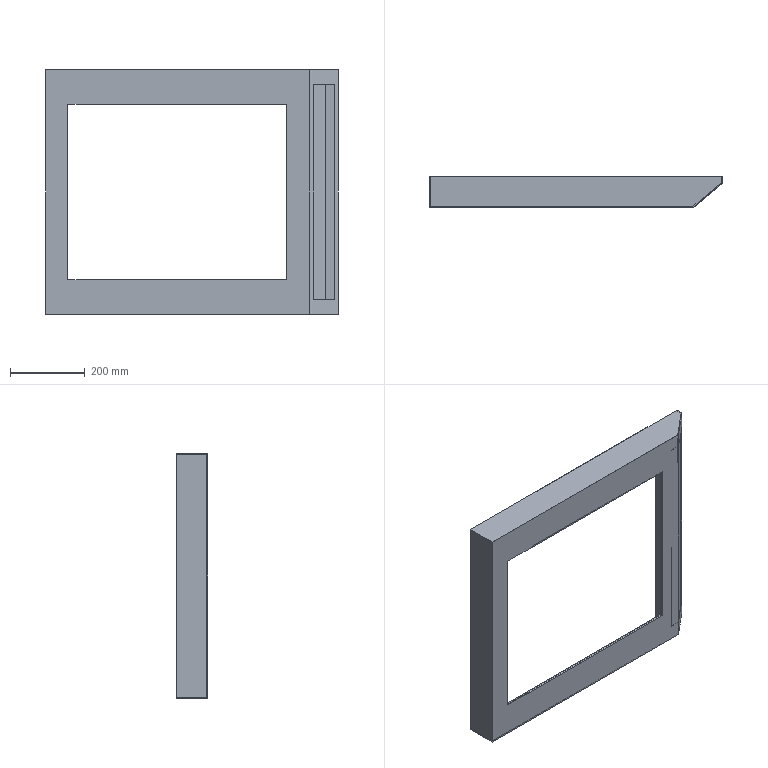Part | SolidWorks | features ICE 9, Extrusion 1, Shell 1 | 4 solids | 60 faces | box 782 x 83 x 654 mm | volume 1247436 mm3 | plane 60